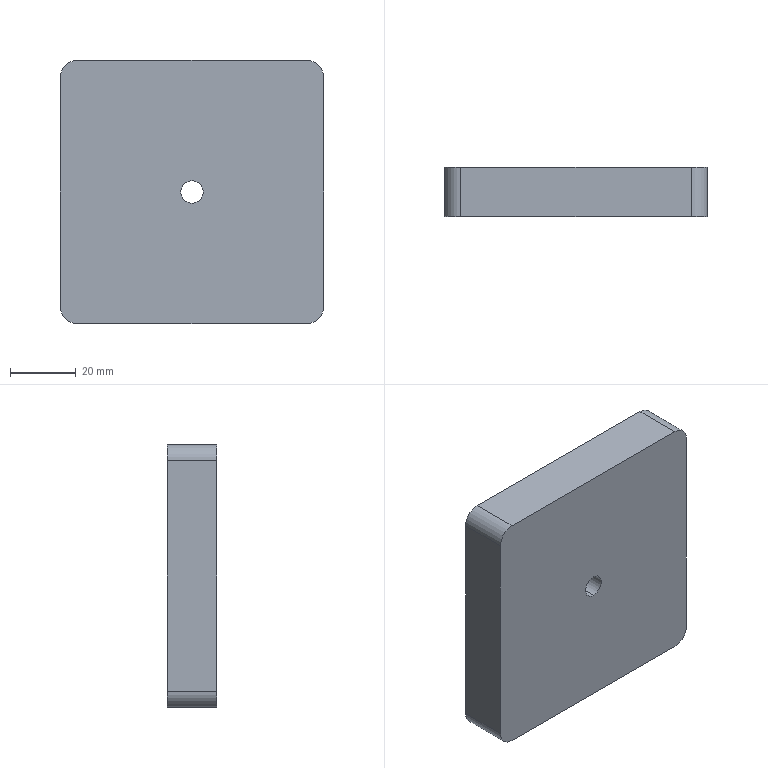Part | SolidWorks | features Extrusion 1, Fillet 1, HoleWzd 1 | 1 solid | 12 faces | box 80 x 15 x 80 mm | volume 95133 mm3 | cylinder 6 | plane 6 | commonest cylinder face diameters 10 x4 6.8 x2
STEP:
#1=CARTESIAN_POINT('',(0.,15.,-3.4));
#2=VERTEX_POINT('',#1);
#3=CARTESIAN_POINT('',(0.,15.,3.4));
#4=VERTEX_POINT('',#3);
#5=CARTESIAN_POINT('',(0.,15.,0.));
#6=DIRECTION('',(0.,1.,0.));
#7=DIRECTION('',(0.,0.,1.));
#8=AXIS2_PLACEMENT_3D('',#5,#6,#7);
#9=CIRCLE('',#8,3.4);
#10=EDGE_CURVE('',#2,#4,#9,.T.);
#11=ORIENTED_EDGE('',*,*,#10,.T.);
#12=CARTESIAN_POINT('',(0.,0.,3.4));
#13=VERTEX_POINT('',#12);
#14=CARTESIAN_POINT('',(0.,0.,3.4));
#15=DIRECTION('',(0.,-1.,0.));
#16=VECTOR('',#15,1000.);
#17=LINE('',#14,#16);
#18=EDGE_CURVE('',#4,#13,#17,.T.);
#19=ORIENTED_EDGE('',*,*,#18,.T.);
#20=CARTESIAN_POINT('',(0.,0.,-3.4));
#21=VERTEX_POINT('',#20);
#22=CARTESIAN_POINT('',(0.,0.,0.));
#23=DIRECTION('',(0.,-1.,0.));
#24=DIRECTION('',(0.,0.,-1.));
#25=AXIS2_PLACEMENT_3D('',#22,#23,#24);
#26=CIRCLE('',#25,3.4);
#27=EDGE_CURVE('',#13,#21,#26,.T.);
#28=ORIENTED_EDGE('',*,*,#27,.T.);
#29=CARTESIAN_POINT('',(0.,0.,-3.4));
#30=DIRECTION('',(0.,-1.,0.));
#31=VECTOR('',#30,1000.);
#32=LINE('',#29,#31);
#33=EDGE_CURVE('',#2,#21,#32,.T.);
#34=ORIENTED_EDGE('',*,*,#33,.F.);
#35=EDGE_LOOP('',(#11,#19,#28,#34));
#36=FACE_OUTER_BOUND('',#35,.T.);
#37=CARTESIAN_POINT('',(0.,0.,0.));
#38=DIRECTION('',(0.,-1.,0.));
#39=DIRECTION('',(0.,0.,-1.));
#40=AXIS2_PLACEMENT_3D('',#37,#38,#39);
#41=CYLINDRICAL_SURFACE('',#40,3.4);
#42=ADVANCED_FACE('',(#36),#41,.F.);
#43=CARTESIAN_POINT('',(40.,15.,35.));
#44=VERTEX_POINT('',#43);
#45=CARTESIAN_POINT('',(40.,15.,-35.));
#46=VERTEX_POINT('',#45);
#47=CARTESIAN_POINT('',(40.,15.,-40.));
#48=DIRECTION('',(0.,0.,-1.));
#49=VECTOR('',#48,1000.);
#50=LINE('',#47,#49);
#51=EDGE_CURVE('',#44,#46,#50,.T.);
#52=ORIENTED_EDGE('',*,*,#51,.F.);
#53=CARTESIAN_POINT('',(40.,0.,35.));
#54=VERTEX_POINT('',#53);
#55=CARTESIAN_POINT('',(40.,15.,35.));
#56=DIRECTION('',(0.,-1.,0.));
#57=VECTOR('',#56,1000.);
#58=LINE('',#55,#57);
#59=EDGE_CURVE('',#44,#54,#58,.T.);
#60=ORIENTED_EDGE('',*,*,#59,.T.);
#61=CARTESIAN_POINT('',(40.,0.,-35.));
#62=VERTEX_POINT('',#61);
#63=CARTESIAN_POINT('',(40.,0.,-40.));
#64=DIRECTION('',(0.,0.,-1.));
#65=VECTOR('',#64,1000.);
#66=LINE('',#63,#65);
#67=EDGE_CURVE('',#54,#62,#66,.T.);
#68=ORIENTED_EDGE('',*,*,#67,.T.);
#69=CARTESIAN_POINT('',(40.,15.,-35.));
#70=DIRECTION('',(0.,1.,0.));
#71=VECTOR('',#70,1000.);
#72=LINE('',#69,#71);
#73=EDGE_CURVE('',#62,#46,#72,.T.);
#74=ORIENTED_EDGE('',*,*,#73,.T.);
#75=EDGE_LOOP('',(#52,#60,#68,#74));
#76=FACE_OUTER_BOUND('',#75,.T.);
#77=CARTESIAN_POINT('',(40.,15.,-40.));
#78=DIRECTION('',(-1.,0.,0.));
#79=DIRECTION('',(0.,0.,1.));
#80=AXIS2_PLACEMENT_3D('',#77,#78,#79);
#81=PLANE('',#80);
#82=ADVANCED_FACE('',(#76),#81,.F.);
#83=CARTESIAN_POINT('',(35.,15.,-40.));
#84=VERTEX_POINT('',#83);
#85=CARTESIAN_POINT('',(-35.,15.,-40.));
#86=VERTEX_POINT('',#85);
#87=CARTESIAN_POINT('',(-40.,15.,-40.));
#88=DIRECTION('',(-1.,0.,0.));
#89=VECTOR('',#88,1000.);
#90=LINE('',#87,#89);
#91=EDGE_CURVE('',#84,#86,#90,.T.);
#92=ORIENTED_EDGE('',*,*,#91,.F.);
#93=CARTESIAN_POINT('',(35.,0.,-40.));
#94=VERTEX_POINT('',#93);
#95=CARTESIAN_POINT('',(35.,15.,-40.));
#96=DIRECTION('',(0.,-1.,0.));
#97=VECTOR('',#96,1000.);
#98=LINE('',#95,#97);
#99=EDGE_CURVE('',#84,#94,#98,.T.);
#100=ORIENTED_EDGE('',*,*,#99,.T.);
#101=CARTESIAN_POINT('',(-35.,0.,-40.));
#102=VERTEX_POINT('',#101);
#103=CARTESIAN_POINT('',(-40.,0.,-40.));
#104=DIRECTION('',(-1.,0.,0.));
#105=VECTOR('',#104,1000.);
#106=LINE('',#103,#105);
#107=EDGE_CURVE('',#94,#102,#106,.T.);
#108=ORIENTED_EDGE('',*,*,#107,.T.);
#109=CARTESIAN_POINT('',(-35.,15.,-40.));
#110=DIRECTION('',(0.,1.,0.));
#111=VECTOR('',#110,1000.);
#112=LINE('',#109,#111);
#113=EDGE_CURVE('',#102,#86,#112,.T.);
#114=ORIENTED_EDGE('',*,*,#113,.T.);
#115=EDGE_LOOP('',(#92,#100,#108,#114));
#116=FACE_OUTER_BOUND('',#115,.T.);
#117=CARTESIAN_POINT('',(-40.,15.,-40.));
#118=DIRECTION('',(0.,0.,1.));
#119=DIRECTION('',(1.,0.,0.));
#120=AXIS2_PLACEMENT_3D('',#117,#118,#119);
#121=PLANE('',#120);
#122=ADVANCED_FACE('',(#116),#121,.F.);
#123=CARTESIAN_POINT('',(-40.,0.,-35.));
#124=VERTEX_POINT('',#123);
#125=CARTESIAN_POINT('',(-40.,0.,35.));
#126=VERTEX_POINT('',#125);
#127=CARTESIAN_POINT('',(-40.,0.,-40.));
#128=DIRECTION('',(0.,0.,1.));
#129=VECTOR('',#128,1000.);
#130=LINE('',#127,#129);
#131=EDGE_CURVE('',#124,#126,#130,.T.);
#132=ORIENTED_EDGE('',*,*,#131,.T.);
#133=CARTESIAN_POINT('',(-40.,15.,35.));
#134=VERTEX_POINT('',#133);
#135=CARTESIAN_POINT('',(-40.,15.,35.));
#136=DIRECTION('',(0.,1.,0.));
#137=VECTOR('',#136,1000.);
#138=LINE('',#135,#137);
#139=EDGE_CURVE('',#126,#134,#138,.T.);
#140=ORIENTED_EDGE('',*,*,#139,.T.);
#141=CARTESIAN_POINT('',(-40.,15.,-35.));
#142=VERTEX_POINT('',#141);
#143=CARTESIAN_POINT('',(-40.,15.,-40.));
#144=DIRECTION('',(0.,0.,1.));
#145=VECTOR('',#144,1000.);
#146=LINE('',#143,#145);
#147=EDGE_CURVE('',#142,#134,#146,.T.);
#148=ORIENTED_EDGE('',*,*,#147,.F.);
#149=CARTESIAN_POINT('',(-40.,15.,-35.));
#150=DIRECTION('',(0.,-1.,0.));
#151=VECTOR('',#150,1000.);
#152=LINE('',#149,#151);
#153=EDGE_CURVE('',#142,#124,#152,.T.);
#154=ORIENTED_EDGE('',*,*,#153,.T.);
#155=EDGE_LOOP('',(#132,#140,#148,#154));
#156=FACE_OUTER_BOUND('',#155,.T.);
#157=CARTESIAN_POINT('',(-40.,15.,-40.));
#158=DIRECTION('',(1.,0.,0.));
#159=DIRECTION('',(0.,0.,-1.));
#160=AXIS2_PLACEMENT_3D('',#157,#158,#159);
#161=PLANE('',#160);
#162=ADVANCED_FACE('',(#156),#161,.F.);
#163=CARTESIAN_POINT('',(-35.,15.,40.));
#164=VERTEX_POINT('',#163);
#165=CARTESIAN_POINT('',(35.,15.,40.));
#166=VERTEX_POINT('',#165);
#167=CARTESIAN_POINT('',(-40.,15.,40.));
#168=DIRECTION('',(1.,0.,0.));
#169=VECTOR('',#168,1000.);
#170=LINE('',#167,#169);
#171=EDGE_CURVE('',#164,#166,#170,.T.);
#172=ORIENTED_EDGE('',*,*,#171,.F.);
#173=CARTESIAN_POINT('',(-35.,0.,40.));
#174=VERTEX_POINT('',#173);
#175=CARTESIAN_POINT('',(-35.,15.,40.));
#176=DIRECTION('',(0.,-1.,0.));
#177=VECTOR('',#176,1000.);
#178=LINE('',#175,#177);
#179=EDGE_CURVE('',#164,#174,#178,.T.);
#180=ORIENTED_EDGE('',*,*,#179,.T.);
#181=CARTESIAN_POINT('',(35.,0.,40.));
#182=VERTEX_POINT('',#181);
#183=CARTESIAN_POINT('',(-40.,0.,40.));
#184=DIRECTION('',(1.,0.,0.));
#185=VECTOR('',#184,1000.);
#186=LINE('',#183,#185);
#187=EDGE_CURVE('',#174,#182,#186,.T.);
#188=ORIENTED_EDGE('',*,*,#187,.T.);
#189=CARTESIAN_POINT('',(35.,15.,40.));
#190=DIRECTION('',(0.,1.,0.));
#191=VECTOR('',#190,1000.);
#192=LINE('',#189,#191);
#193=EDGE_CURVE('',#182,#166,#192,.T.);
#194=ORIENTED_EDGE('',*,*,#193,.T.);
#195=EDGE_LOOP('',(#172,#180,#188,#194));
#196=FACE_OUTER_BOUND('',#195,.T.);
#197=CARTESIAN_POINT('',(-40.,15.,40.));
#198=DIRECTION('',(0.,0.,-1.));
#199=DIRECTION('',(-1.,0.,0.));
#200=AXIS2_PLACEMENT_3D('',#197,#198,#199);
#201=PLANE('',#200);
#202=ADVANCED_FACE('',(#196),#201,.F.);
#203=ORIENTED_EDGE('',*,*,#10,.F.);
#204=CARTESIAN_POINT('',(0.,15.,0.));
#205=DIRECTION('',(0.,1.,0.));
#206=DIRECTION('',(0.,0.,1.));
#207=AXIS2_PLACEMENT_3D('',#204,#205,#206);
#208=CIRCLE('',#207,3.4);
#209=EDGE_CURVE('',#4,#2,#208,.T.);
#210=ORIENTED_EDGE('',*,*,#209,.F.);
#211=EDGE_LOOP('',(#203,#210));
#212=FACE_BOUND('',#211,.T.);
#213=ORIENTED_EDGE('',*,*,#147,.T.);
#214=CARTESIAN_POINT('',(-35.,15.,35.));
#215=DIRECTION('',(0.,1.,0.));
#216=DIRECTION('',(0.,0.,1.));
#217=AXIS2_PLACEMENT_3D('',#214,#215,#216);
#218=CIRCLE('',#217,5.);
#219=EDGE_CURVE('',#134,#164,#218,.T.);
#220=ORIENTED_EDGE('',*,*,#219,.T.);
#221=ORIENTED_EDGE('',*,*,#171,.T.);
#222=CARTESIAN_POINT('',(35.,15.,35.));
#223=DIRECTION('',(0.,1.,0.));
#224=DIRECTION('',(0.,0.,1.));
#225=AXIS2_PLACEMENT_3D('',#222,#223,#224);
#226=CIRCLE('',#225,5.);
#227=EDGE_CURVE('',#166,#44,#226,.T.);
#228=ORIENTED_EDGE('',*,*,#227,.T.);
#229=ORIENTED_EDGE('',*,*,#51,.T.);
#230=CARTESIAN_POINT('',(35.,15.,-35.));
#231=DIRECTION('',(0.,1.,0.));
#232=DIRECTION('',(0.,0.,1.));
#233=AXIS2_PLACEMENT_3D('',#230,#231,#232);
#234=CIRCLE('',#233,5.);
#235=EDGE_CURVE('',#46,#84,#234,.T.);
#236=ORIENTED_EDGE('',*,*,#235,.T.);
#237=ORIENTED_EDGE('',*,*,#91,.T.);
#238=CARTESIAN_POINT('',(-35.,15.,-35.));
#239=DIRECTION('',(0.,1.,0.));
#240=DIRECTION('',(0.,0.,1.));
#241=AXIS2_PLACEMENT_3D('',#238,#239,#240);
#242=CIRCLE('',#241,5.);
#243=EDGE_CURVE('',#86,#142,#242,.T.);
#244=ORIENTED_EDGE('',*,*,#243,.T.);
#245=EDGE_LOOP('',(#213,#220,#221,#228,#229,#236,#237,#244));
#246=FACE_OUTER_BOUND('',#245,.T.);
#247=CARTESIAN_POINT('',(0.,15.,0.));
#248=DIRECTION('',(0.,1.,0.));
#249=DIRECTION('',(0.,0.,1.));
#250=AXIS2_PLACEMENT_3D('',#247,#248,#249);
#251=PLANE('',#250);
#252=ADVANCED_FACE('',(#212,#246),#251,.T.);
#253=CARTESIAN_POINT('',(0.,0.,0.));
#254=DIRECTION('',(0.,-1.,0.));
#255=DIRECTION('',(0.,0.,-1.));
#256=AXIS2_PLACEMENT_3D('',#253,#254,#255);
#257=CIRCLE('',#256,3.4);
#258=EDGE_CURVE('',#21,#13,#257,.T.);
#259=ORIENTED_EDGE('',*,*,#258,.F.);
#260=ORIENTED_EDGE('',*,*,#27,.F.);
#261=EDGE_LOOP('',(#259,#260));
#262=FACE_BOUND('',#261,.T.);
#263=ORIENTED_EDGE('',*,*,#187,.F.);
#264=CARTESIAN_POINT('',(-35.,0.,35.));
#265=DIRECTION('',(0.,-1.,0.));
#266=DIRECTION('',(0.,0.,1.));
#267=AXIS2_PLACEMENT_3D('',#264,#265,#266);
#268=CIRCLE('',#267,5.);
#269=EDGE_CURVE('',#174,#126,#268,.T.);
#270=ORIENTED_EDGE('',*,*,#269,.T.);
#271=ORIENTED_EDGE('',*,*,#131,.F.);
#272=CARTESIAN_POINT('',(-35.,0.,-35.));
#273=DIRECTION('',(0.,-1.,0.));
#274=DIRECTION('',(0.,0.,1.));
#275=AXIS2_PLACEMENT_3D('',#272,#273,#274);
#276=CIRCLE('',#275,5.);
#277=EDGE_CURVE('',#124,#102,#276,.T.);
#278=ORIENTED_EDGE('',*,*,#277,.T.);
#279=ORIENTED_EDGE('',*,*,#107,.F.);
#280=CARTESIAN_POINT('',(35.,0.,-35.));
#281=DIRECTION('',(0.,-1.,0.));
#282=DIRECTION('',(0.,0.,1.));
#283=AXIS2_PLACEMENT_3D('',#280,#281,#282);
#284=CIRCLE('',#283,5.);
#285=EDGE_CURVE('',#94,#62,#284,.T.);
#286=ORIENTED_EDGE('',*,*,#285,.T.);
#287=ORIENTED_EDGE('',*,*,#67,.F.);
#288=CARTESIAN_POINT('',(35.,0.,35.));
#289=DIRECTION('',(0.,-1.,0.));
#290=DIRECTION('',(0.,0.,1.));
#291=AXIS2_PLACEMENT_3D('',#288,#289,#290);
#292=CIRCLE('',#291,5.);
#293=EDGE_CURVE('',#54,#182,#292,.T.);
#294=ORIENTED_EDGE('',*,*,#293,.T.);
#295=EDGE_LOOP('',(#263,#270,#271,#278,#279,#286,#287,#294));
#296=FACE_OUTER_BOUND('',#295,.T.);
#297=CARTESIAN_POINT('',(0.,0.,0.));
#298=DIRECTION('',(0.,1.,0.));
#299=DIRECTION('',(0.,0.,1.));
#300=AXIS2_PLACEMENT_3D('',#297,#298,#299);
#301=PLANE('',#300);
#302=ADVANCED_FACE('',(#262,#296),#301,.F.);
#303=ORIENTED_EDGE('',*,*,#219,.F.);
#304=ORIENTED_EDGE('',*,*,#139,.F.);
#305=ORIENTED_EDGE('',*,*,#269,.F.);
#306=ORIENTED_EDGE('',*,*,#179,.F.);
#307=EDGE_LOOP('',(#303,#304,#305,#306));
#308=FACE_OUTER_BOUND('',#307,.T.);
#309=CARTESIAN_POINT('',(-35.,15.,35.));
#310=DIRECTION('',(0.,-1.,0.));
#311=DIRECTION('',(0.,0.,-1.));
#312=AXIS2_PLACEMENT_3D('',#309,#310,#311);
#313=CYLINDRICAL_SURFACE('',#312,5.);
#314=ADVANCED_FACE('',(#308),#313,.T.);
#315=ORIENTED_EDGE('',*,*,#227,.F.);
#316=ORIENTED_EDGE('',*,*,#193,.F.);
#317=ORIENTED_EDGE('',*,*,#293,.F.);
#318=ORIENTED_EDGE('',*,*,#59,.F.);
#319=EDGE_LOOP('',(#315,#316,#317,#318));
#320=FACE_OUTER_BOUND('',#319,.T.);
#321=CARTESIAN_POINT('',(35.,15.,35.));
#322=DIRECTION('',(0.,-1.,0.));
#323=DIRECTION('',(0.,0.,-1.));
#324=AXIS2_PLACEMENT_3D('',#321,#322,#323);
#325=CYLINDRICAL_SURFACE('',#324,5.);
#326=ADVANCED_FACE('',(#320),#325,.T.);
#327=ORIENTED_EDGE('',*,*,#235,.F.);
#328=ORIENTED_EDGE('',*,*,#73,.F.);
#329=ORIENTED_EDGE('',*,*,#285,.F.);
#330=ORIENTED_EDGE('',*,*,#99,.F.);
#331=EDGE_LOOP('',(#327,#328,#329,#330));
#332=FACE_OUTER_BOUND('',#331,.T.);
#333=CARTESIAN_POINT('',(35.,15.,-35.));
#334=DIRECTION('',(0.,-1.,0.));
#335=DIRECTION('',(0.,0.,-1.));
#336=AXIS2_PLACEMENT_3D('',#333,#334,#335);
#337=CYLINDRICAL_SURFACE('',#336,5.);
#338=ADVANCED_FACE('',(#332),#337,.T.);
#339=ORIENTED_EDGE('',*,*,#243,.F.);
#340=ORIENTED_EDGE('',*,*,#113,.F.);
#341=ORIENTED_EDGE('',*,*,#277,.F.);
#342=ORIENTED_EDGE('',*,*,#153,.F.);
#343=EDGE_LOOP('',(#339,#340,#341,#342));
#344=FACE_OUTER_BOUND('',#343,.T.);
#345=CARTESIAN_POINT('',(-35.,15.,-35.));
#346=DIRECTION('',(0.,-1.,0.));
#347=DIRECTION('',(0.,0.,-1.));
#348=AXIS2_PLACEMENT_3D('',#345,#346,#347);
#349=CYLINDRICAL_SURFACE('',#348,5.);
#350=ADVANCED_FACE('',(#344),#349,.T.);
#351=ORIENTED_EDGE('',*,*,#18,.F.);
#352=ORIENTED_EDGE('',*,*,#209,.T.);
#353=ORIENTED_EDGE('',*,*,#33,.T.);
#354=ORIENTED_EDGE('',*,*,#258,.T.);
#355=EDGE_LOOP('',(#351,#352,#353,#354));
#356=FACE_OUTER_BOUND('',#355,.T.);
#357=CARTESIAN_POINT('',(0.,0.,0.));
#358=DIRECTION('',(0.,-1.,0.));
#359=DIRECTION('',(0.,0.,-1.));
#360=AXIS2_PLACEMENT_3D('',#357,#358,#359);
#361=CYLINDRICAL_SURFACE('',#360,3.4);
#362=ADVANCED_FACE('',(#356),#361,.F.);
#363=CLOSED_SHELL('',(#42,#82,#122,#162,#202,#252,#302,#314,#326,#338,#350,#362));
#364=MANIFOLD_SOLID_BREP('',#363);
#365=CARTESIAN_POINT('',(0.,0.,0.));
#366=DIRECTION('',(0.,0.,1.));
#367=DIRECTION('',(1.,0.,0.));
#368=AXIS2_PLACEMENT_3D('',#365,#366,#367);
#369=(LENGTH_UNIT()NAMED_UNIT(*)SI_UNIT(.MILLI.,.METRE.));
#370=UNCERTAINTY_MEASURE_WITH_UNIT(LENGTH_MEASURE(0.00001),#369,'','');
#371=(NAMED_UNIT(*)PLANE_ANGLE_UNIT()SI_UNIT($,.RADIAN.));
#372=(NAMED_UNIT(*)SI_UNIT($,.STERADIAN.)SOLID_ANGLE_UNIT());
#373=(GEOMETRIC_REPRESENTATION_CONTEXT(3)GLOBAL_UNCERTAINTY_ASSIGNED_CONTEXT((#370))GLOBAL_UNIT_ASSIGNED_CONTEXT((#369,#371,#372))REPRESENTATION_CONTEXT('',''));
#374=ADVANCED_BREP_SHAPE_REPRESENTATION('',(#364,#368),#373);